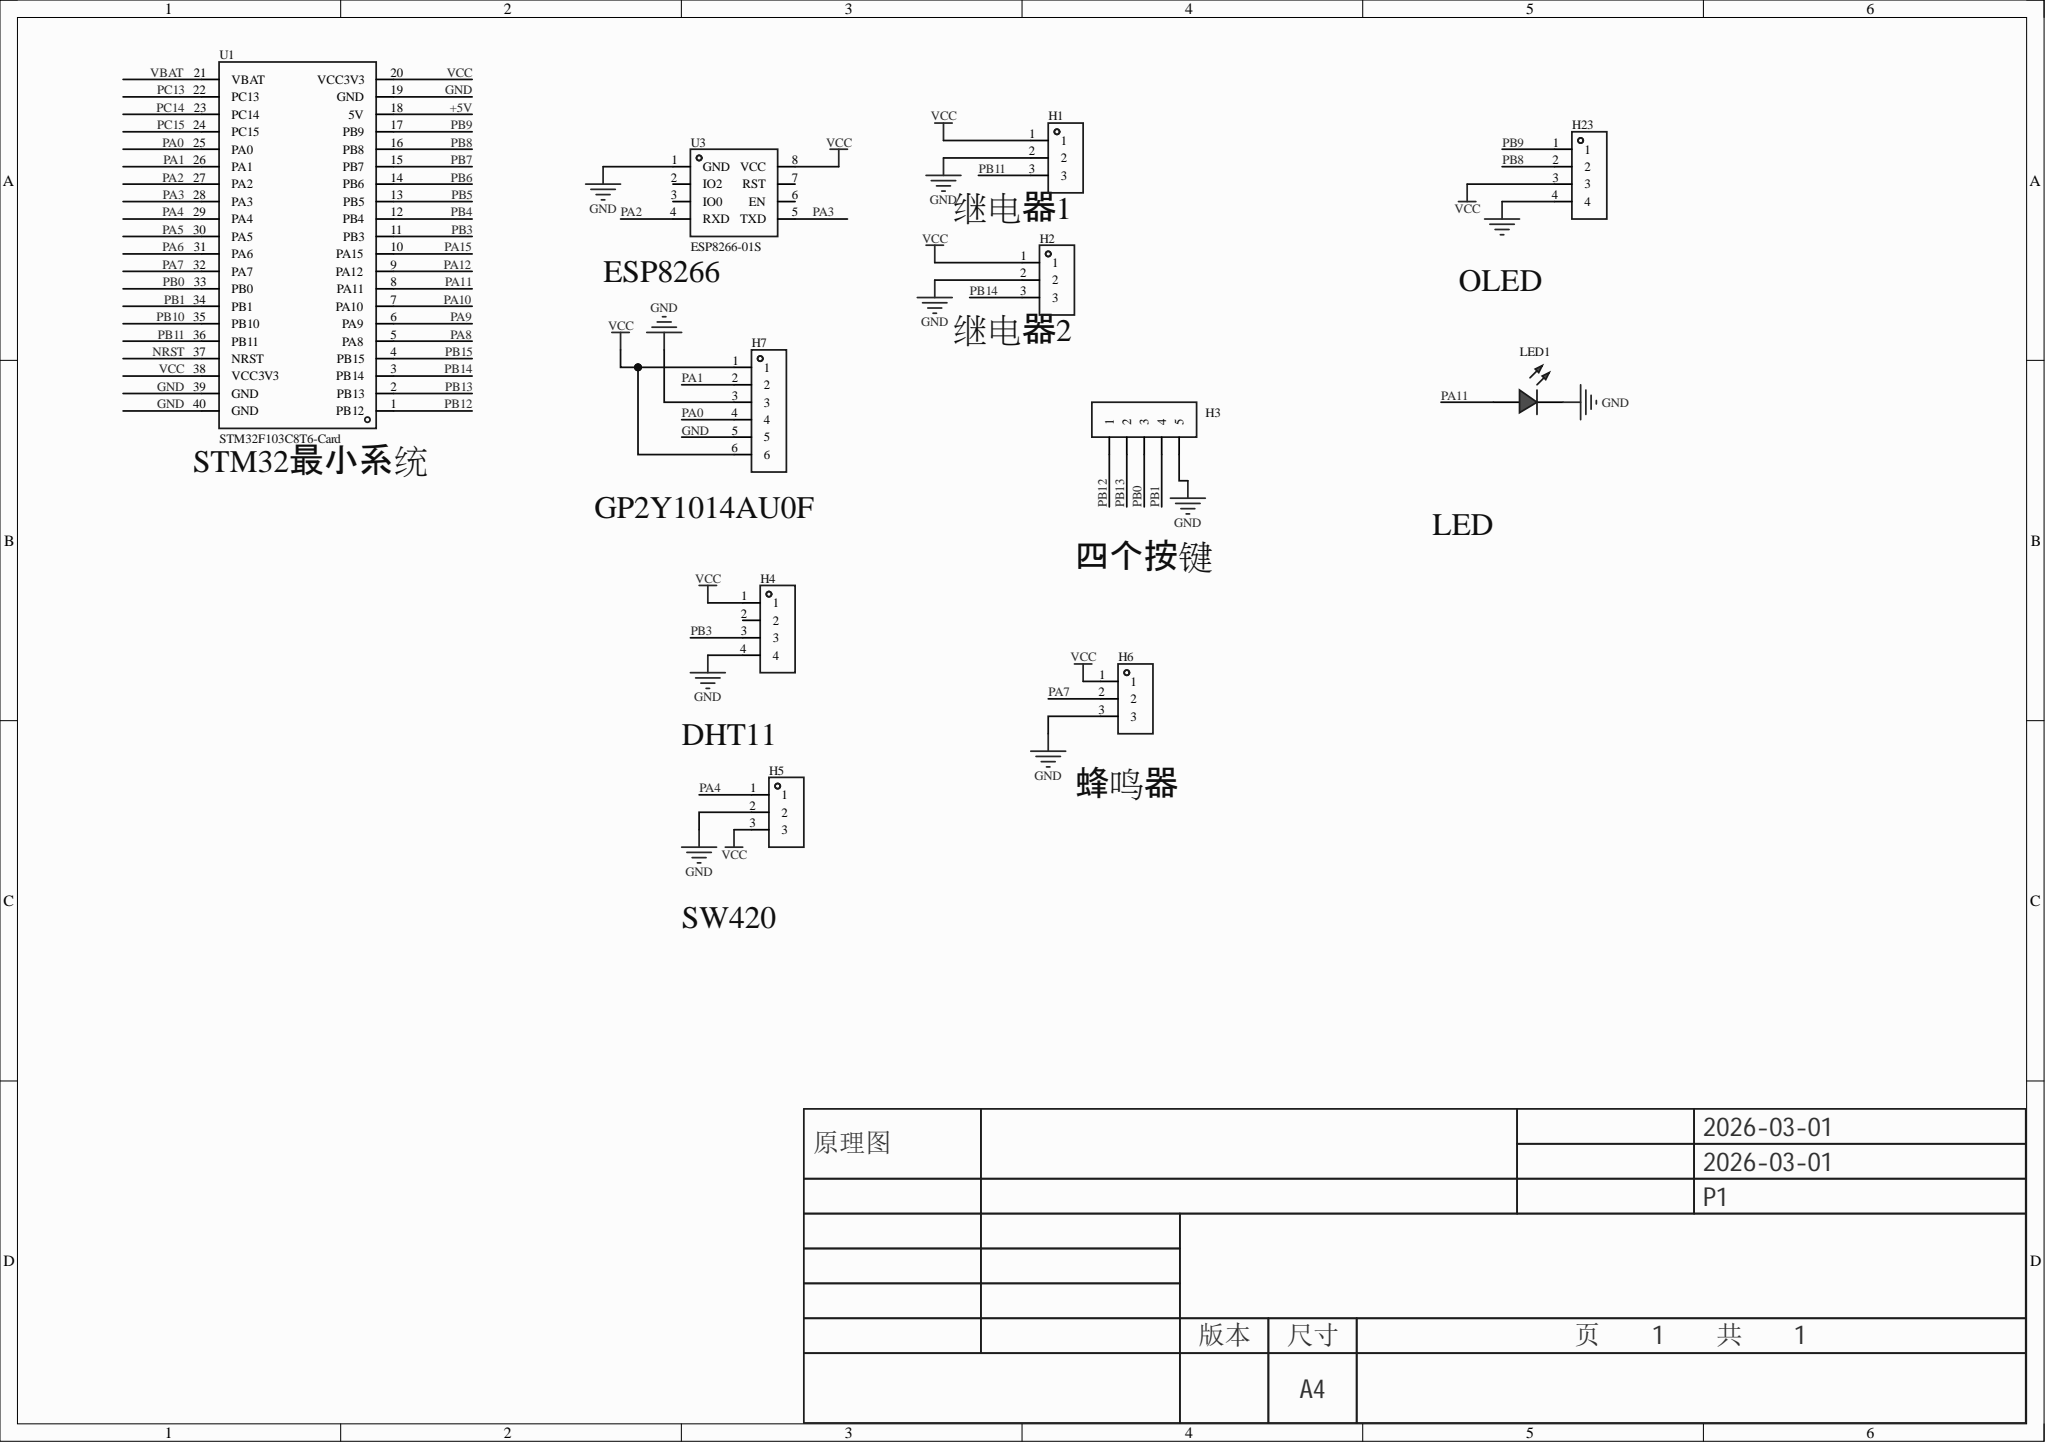Circuit board | Altium Designer | 11 parts | 18 nets
Bill of materials:
Comment,Description,Designator,Footprint,LibRef,Quantity
"","","H1, H2, H5, H6","HDR-TH_3P-P2.54-V-F","HDR-F_2.54_1x3P","4"
"","","H3","HDR-TH_5P-P2.54-V-F","HDR-F_2.54_1x5P","1"
"","","H4, H23","HDR-TH_4P-P2.54-V-F","HDR-F_2.54_1x4P","2"
"","","H7","HDR-TH_6P-P2.54-V-F","HDR-F_2.54_1x6P","1"
"","","LED1","LED_TH-3mm","LED_TH-R_3mm","1"
"STM32F103C8T6-Card","","U1","CONN-TH_L53.3-W22.9_STM32F103C8T6-CARD","STM32F103C8T6-Card","1"
"ESP8266-01S","","U3","WIFIM-TH_ESP8266-01S","ESP8266-01S","1"
Netlist (Protel format):
[
H1
HDR-TH_3P-P2.54-V-F




]
[
H2
HDR-TH_3P-P2.54-V-F




]
[
H3
HDR-TH_5P-P2.54-V-F




]
[
H4
HDR-TH_4P-P2.54-V-F




]
[
H5
HDR-TH_3P-P2.54-V-F




]
[
H6
HDR-TH_3P-P2.54-V-F




]
[
H7
HDR-TH_6P-P2.54-V-F




]
[
H23
HDR-TH_4P-P2.54-V-F




]
[
LED1
LED_TH-3mm




]
[
U1
CONN-TH_L53.3-W22.9_STM32F103C8T6-CARD
STM32F103C8T6-Card



]
[
U3
WIFIM-TH_ESP8266-01S
ESP8266-01S



]
(
VCC
H1-1
H2-1
H4-1
H5-3
H6-1
H7-1
H7-6
H23-3
U1-20
U1-38
U3-8
)
(
PB14
H2-3
U1-3
)
(
PB13
H3-2
U1-2
)
(
PB12
H3-1
U1-1
)
(
PB11
H1-3
U1-36
)
(
PB9
H23-1
U1-17
)
(
PB8
H23-2
U1-16
)
(
PB3
H4-3
U1-11
)
(
PB1
H3-4
U1-34
)
(
PB0
H3-3
U1-33
)
(
PA11
LED1-1
U1-8
)
(
PA7
H6-2
U1-32
)
(
PA4
H5-1
U1-29
)
(
PA3
U1-28
U3-5
)
(
PA2
U1-27
U3-4
)
(
PA1
H7-2
U1-26
)
(
PA0
H7-4
U1-25
)
(
GND
H1-2
H2-2
H3-5
H4-4
H5-2
H6-3
H7-3
H7-5
H23-4
LED1-2
U1-19
U1-39
U1-40
U3-1
)